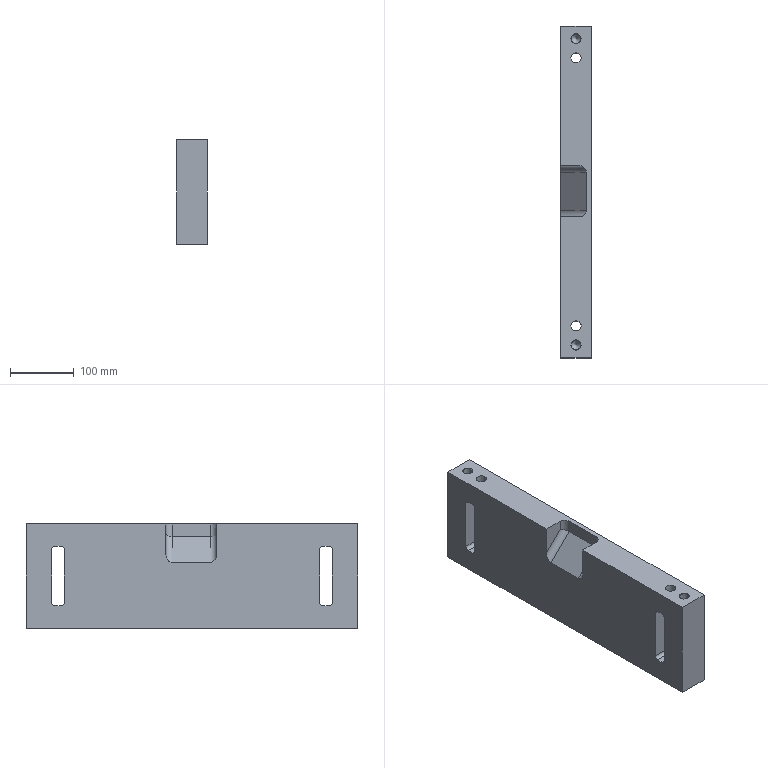Part | NX | features B2-7 2 | 1 solid | 50 faces | box 48 x 520 x 163 mm | volume 3697198 mm3 | plane 22 | cylinder 20 | cone 8 | commonest cylinder face diameters 10 x8 14.506 x4 16 x4 20 x4